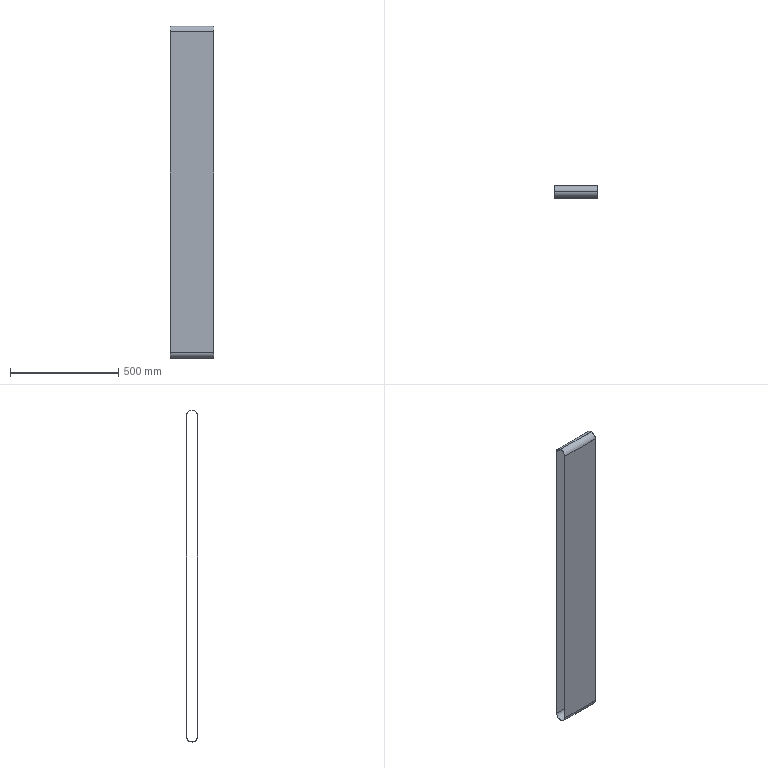Part | STEP file | 02-15 Conveyor belt | 1 solid | 12 faces | box 200 x 54 x 1534 mm | volume 1249345 mm3 | cylinder 6 | plane 6 | commonest cylinder face diameters 50 x3 54 x3
STEP:
#1=CARTESIAN_POINT('',(0.,0.,0.));
#2=DIRECTION('',(0.,0.,1.));
#3=DIRECTION('',(1.,0.,0.));
#4=AXIS2_PLACEMENT_3D('',#1,#2,#3);
#5=CARTESIAN_POINT('',(-100.,25.,740.));
#6=VERTEX_POINT('',#5);
#7=CARTESIAN_POINT('',(100.,25.,740.));
#8=VERTEX_POINT('',#7);
#9=CARTESIAN_POINT('',(0.,25.,740.));
#10=DIRECTION('',(1.,0.,0.));
#11=VECTOR('',#10,1.);
#12=LINE('',#9,#11);
#13=CARTESIAN_POINT('',(100.,0.,740.));
#14=DIRECTION('',(-1.,0.,0.));
#15=DIRECTION('',(0.,0.,1.));
#16=AXIS2_PLACEMENT_3D('',#13,#14,#15);
#17=CYLINDRICAL_SURFACE('',#16,25.);
#18=CARTESIAN_POINT('',(1.571,100.));
#19=DIRECTION('',(0.,-1.));
#20=VECTOR('',#19,1.);
#21=LINE('',#18,#20);
#22=(GEOMETRIC_REPRESENTATION_CONTEXT(2)PARAMETRIC_REPRESENTATION_CONTEXT()REPRESENTATION_CONTEXT('',''));
#23=DEFINITIONAL_REPRESENTATION('',(#21),#22);
#24=PCURVE('',#17,#23);
#25=CARTESIAN_POINT('',(-100.,25.,740.));
#26=DIRECTION('',(0.,-1.,0.));
#27=DIRECTION('',(0.,0.,-1.));
#28=AXIS2_PLACEMENT_3D('',#25,#26,#27);
#29=PLANE('',#28);
#30=CARTESIAN_POINT('',(0.000000005,100.));
#31=DIRECTION('',(0.,1.));
#32=VECTOR('',#31,1.);
#33=LINE('',#30,#32);
#34=(GEOMETRIC_REPRESENTATION_CONTEXT(2)PARAMETRIC_REPRESENTATION_CONTEXT()REPRESENTATION_CONTEXT('',''));
#35=DEFINITIONAL_REPRESENTATION('',(#33),#34);
#36=PCURVE('',#29,#35);
#37=SURFACE_CURVE('',#12,(#24,#36),.PCURVE_S1.);
#38=EDGE_CURVE('',#6,#8,#37,.T.);
#39=ORIENTED_EDGE('',*,*,#38,.F.);
#40=CARTESIAN_POINT('',(-100.,0.,765.));
#41=VERTEX_POINT('',#40);
#42=CARTESIAN_POINT('',(-100.,0.,740.));
#43=DIRECTION('',(-1.,0.,0.));
#44=DIRECTION('',(0.,0.,1.));
#45=AXIS2_PLACEMENT_3D('',#42,#43,#44);
#46=CIRCLE('',#45,25.);
#47=CARTESIAN_POINT('',(0.,200.));
#48=DIRECTION('',(1.,0.));
#49=VECTOR('',#48,1.);
#50=LINE('',#47,#49);
#51=(GEOMETRIC_REPRESENTATION_CONTEXT(2)PARAMETRIC_REPRESENTATION_CONTEXT()REPRESENTATION_CONTEXT('',''));
#52=DEFINITIONAL_REPRESENTATION('',(#50),#51);
#53=PCURVE('',#17,#52);
#54=CARTESIAN_POINT('',(-100.,-27.,776.204));
#55=DIRECTION('',(1.,0.,0.));
#56=DIRECTION('',(0.,0.,-1.));
#57=AXIS2_PLACEMENT_3D('',#54,#55,#56);
#58=PLANE('',#57);
#59=CARTESIAN_POINT('',(11.204,27.));
#60=CARTESIAN_POINT('',(11.204,70.301));
#61=CARTESIAN_POINT('',(48.704,48.651));
#62=CARTESIAN_POINT('',(86.204,27.));
#63=CARTESIAN_POINT('',(48.704,5.349));
#64=CARTESIAN_POINT('',(11.204,-16.301));
#65=CARTESIAN_POINT('',(11.204,27.));
#66=(BOUNDED_CURVE()B_SPLINE_CURVE(2,(#59,#60,#61,#62,#63,#64,#65),.UNSPECIFIED.,.T.,.F.)B_SPLINE_CURVE_WITH_KNOTS((1,2,2,2,2,1),(-2.094,0.,2.094,4.189,6.283,8.378),.UNSPECIFIED.)CURVE()GEOMETRIC_REPRESENTATION_ITEM()RATIONAL_B_SPLINE_CURVE((1.,0.5,1.,0.5,1.,0.5,1.))REPRESENTATION_ITEM(''));
#67=(GEOMETRIC_REPRESENTATION_CONTEXT(2)PARAMETRIC_REPRESENTATION_CONTEXT()REPRESENTATION_CONTEXT('',''));
#68=DEFINITIONAL_REPRESENTATION('',(#66),#67);
#69=PCURVE('',#58,#68);
#70=SURFACE_CURVE('',#46,(#53,#69),.PCURVE_S1.);
#71=EDGE_CURVE('',#41,#6,#70,.T.);
#72=ORIENTED_EDGE('',*,*,#71,.F.);
#73=CARTESIAN_POINT('',(100.,0.,765.));
#74=VERTEX_POINT('',#73);
#75=CARTESIAN_POINT('',(100.,0.,765.));
#76=DIRECTION('',(-1.,0.,0.));
#77=VECTOR('',#76,1.);
#78=LINE('',#75,#77);
#79=CARTESIAN_POINT('',(0.,0.));
#80=DIRECTION('',(0.,1.));
#81=VECTOR('',#80,1.);
#82=LINE('',#79,#81);
#83=(GEOMETRIC_REPRESENTATION_CONTEXT(2)PARAMETRIC_REPRESENTATION_CONTEXT()REPRESENTATION_CONTEXT('',''));
#84=DEFINITIONAL_REPRESENTATION('',(#82),#83);
#85=PCURVE('',#17,#84);
#86=CARTESIAN_POINT('',(100.,0.,740.));
#87=DIRECTION('',(-1.,0.,0.));
#88=DIRECTION('',(0.,0.,1.));
#89=AXIS2_PLACEMENT_3D('',#86,#87,#88);
#90=CYLINDRICAL_SURFACE('',#89,25.);
#91=CARTESIAN_POINT('',(6.283,0.));
#92=DIRECTION('',(0.,1.));
#93=VECTOR('',#92,1.);
#94=LINE('',#91,#93);
#95=(GEOMETRIC_REPRESENTATION_CONTEXT(2)PARAMETRIC_REPRESENTATION_CONTEXT()REPRESENTATION_CONTEXT('',''));
#96=DEFINITIONAL_REPRESENTATION('',(#94),#95);
#97=PCURVE('',#90,#96);
#98=SURFACE_CURVE('',#78,(#85,#97),.PCURVE_S1.);
#99=EDGE_CURVE('',#74,#41,#98,.T.);
#100=ORIENTED_EDGE('',*,*,#99,.F.);
#101=CARTESIAN_POINT('',(100.,0.,740.));
#102=DIRECTION('',(1.,0.,0.));
#103=DIRECTION('',(0.,0.,1.));
#104=AXIS2_PLACEMENT_3D('',#101,#102,#103);
#105=CIRCLE('',#104,25.);
#106=CARTESIAN_POINT('',(6.283,0.));
#107=DIRECTION('',(-1.,0.));
#108=VECTOR('',#107,1.);
#109=LINE('',#106,#108);
#110=(GEOMETRIC_REPRESENTATION_CONTEXT(2)PARAMETRIC_REPRESENTATION_CONTEXT()REPRESENTATION_CONTEXT('',''));
#111=DEFINITIONAL_REPRESENTATION('',(#109),#110);
#112=PCURVE('',#17,#111);
#113=CARTESIAN_POINT('',(100.,-27.,776.204));
#114=DIRECTION('',(1.,0.,0.));
#115=DIRECTION('',(0.,0.,-1.));
#116=AXIS2_PLACEMENT_3D('',#113,#114,#115);
#117=PLANE('',#116);
#118=CARTESIAN_POINT('',(36.204,27.));
#119=DIRECTION('',(-1.,0.));
#120=AXIS2_PLACEMENT_2D('',#118,#119);
#121=CIRCLE('',#120,25.);
#122=(GEOMETRIC_REPRESENTATION_CONTEXT(2)PARAMETRIC_REPRESENTATION_CONTEXT()REPRESENTATION_CONTEXT('',''));
#123=DEFINITIONAL_REPRESENTATION('',(#121),#122);
#124=PCURVE('',#117,#123);
#125=SURFACE_CURVE('',#105,(#112,#124),.PCURVE_S1.);
#126=EDGE_CURVE('',#8,#74,#125,.T.);
#127=ORIENTED_EDGE('',*,*,#126,.F.);
#128=EDGE_LOOP('',(#39,#72,#100,#127));
#129=FACE_BOUND('',#128,.F.);
#130=ADVANCED_FACE('',(#129),#17,.F.);
#131=CARTESIAN_POINT('',(100.,0.,767.));
#132=VERTEX_POINT('',#131);
#133=CARTESIAN_POINT('',(100.,-27.,740.));
#134=VERTEX_POINT('',#133);
#135=CARTESIAN_POINT('',(100.,0.,740.));
#136=DIRECTION('',(1.,0.,0.));
#137=DIRECTION('',(0.,0.,1.));
#138=AXIS2_PLACEMENT_3D('',#135,#136,#137);
#139=CIRCLE('',#138,27.);
#140=CARTESIAN_POINT('',(100.,0.,740.));
#141=DIRECTION('',(-1.,0.,0.));
#142=DIRECTION('',(0.,0.,1.));
#143=AXIS2_PLACEMENT_3D('',#140,#141,#142);
#144=CYLINDRICAL_SURFACE('',#143,27.);
#145=CARTESIAN_POINT('',(6.283,0.));
#146=DIRECTION('',(-1.,0.));
#147=VECTOR('',#146,1.);
#148=LINE('',#145,#147);
#149=(GEOMETRIC_REPRESENTATION_CONTEXT(2)PARAMETRIC_REPRESENTATION_CONTEXT()REPRESENTATION_CONTEXT('',''));
#150=DEFINITIONAL_REPRESENTATION('',(#148),#149);
#151=PCURVE('',#144,#150);
#152=CARTESIAN_POINT('',(36.204,27.));
#153=DIRECTION('',(-1.,0.));
#154=AXIS2_PLACEMENT_2D('',#152,#153);
#155=CIRCLE('',#154,27.);
#156=(GEOMETRIC_REPRESENTATION_CONTEXT(2)PARAMETRIC_REPRESENTATION_CONTEXT()REPRESENTATION_CONTEXT('',''));
#157=DEFINITIONAL_REPRESENTATION('',(#155),#156);
#158=PCURVE('',#117,#157);
#159=SURFACE_CURVE('',#139,(#151,#158),.PCURVE_S1.);
#160=EDGE_CURVE('',#132,#134,#159,.T.);
#161=ORIENTED_EDGE('',*,*,#160,.F.);
#162=CARTESIAN_POINT('',(-100.,0.,767.));
#163=VERTEX_POINT('',#162);
#164=CARTESIAN_POINT('',(100.,0.,767.));
#165=DIRECTION('',(-1.,0.,0.));
#166=VECTOR('',#165,1.);
#167=LINE('',#164,#166);
#168=CARTESIAN_POINT('',(6.283,0.));
#169=DIRECTION('',(0.,1.));
#170=VECTOR('',#169,1.);
#171=LINE('',#168,#170);
#172=(GEOMETRIC_REPRESENTATION_CONTEXT(2)PARAMETRIC_REPRESENTATION_CONTEXT()REPRESENTATION_CONTEXT('',''));
#173=DEFINITIONAL_REPRESENTATION('',(#171),#172);
#174=PCURVE('',#144,#173);
#175=CARTESIAN_POINT('',(100.,0.,740.));
#176=DIRECTION('',(-1.,0.,0.));
#177=DIRECTION('',(0.,0.,1.));
#178=AXIS2_PLACEMENT_3D('',#175,#176,#177);
#179=CYLINDRICAL_SURFACE('',#178,27.);
#180=CARTESIAN_POINT('',(0.,0.));
#181=DIRECTION('',(0.,1.));
#182=VECTOR('',#181,1.);
#183=LINE('',#180,#182);
#184=(GEOMETRIC_REPRESENTATION_CONTEXT(2)PARAMETRIC_REPRESENTATION_CONTEXT()REPRESENTATION_CONTEXT('',''));
#185=DEFINITIONAL_REPRESENTATION('',(#183),#184);
#186=PCURVE('',#179,#185);
#187=SURFACE_CURVE('',#167,(#174,#186),.PCURVE_S1.);
#188=EDGE_CURVE('',#132,#163,#187,.T.);
#189=ORIENTED_EDGE('',*,*,#188,.T.);
#190=CARTESIAN_POINT('',(-100.,-27.,740.));
#191=VERTEX_POINT('',#190);
#192=CARTESIAN_POINT('',(-100.,0.,740.));
#193=DIRECTION('',(1.,0.,0.));
#194=DIRECTION('',(0.,0.,1.));
#195=AXIS2_PLACEMENT_3D('',#192,#193,#194);
#196=CIRCLE('',#195,27.);
#197=CARTESIAN_POINT('',(6.283,200.));
#198=DIRECTION('',(-1.,0.));
#199=VECTOR('',#198,1.);
#200=LINE('',#197,#199);
#201=(GEOMETRIC_REPRESENTATION_CONTEXT(2)PARAMETRIC_REPRESENTATION_CONTEXT()REPRESENTATION_CONTEXT('',''));
#202=DEFINITIONAL_REPRESENTATION('',(#200),#201);
#203=PCURVE('',#144,#202);
#204=CARTESIAN_POINT('',(36.204,27.));
#205=DIRECTION('',(-1.,0.));
#206=AXIS2_PLACEMENT_2D('',#204,#205);
#207=CIRCLE('',#206,27.);
#208=(GEOMETRIC_REPRESENTATION_CONTEXT(2)PARAMETRIC_REPRESENTATION_CONTEXT()REPRESENTATION_CONTEXT('',''));
#209=DEFINITIONAL_REPRESENTATION('',(#207),#208);
#210=PCURVE('',#58,#209);
#211=SURFACE_CURVE('',#196,(#203,#210),.PCURVE_S1.);
#212=EDGE_CURVE('',#163,#191,#211,.T.);
#213=ORIENTED_EDGE('',*,*,#212,.T.);
#214=CARTESIAN_POINT('',(0.,-27.,740.));
#215=DIRECTION('',(1.,0.,0.));
#216=VECTOR('',#215,1.);
#217=LINE('',#214,#216);
#218=CARTESIAN_POINT('',(4.712,100.));
#219=DIRECTION('',(0.,-1.));
#220=VECTOR('',#219,1.);
#221=LINE('',#218,#220);
#222=(GEOMETRIC_REPRESENTATION_CONTEXT(2)PARAMETRIC_REPRESENTATION_CONTEXT()REPRESENTATION_CONTEXT('',''));
#223=DEFINITIONAL_REPRESENTATION('',(#221),#222);
#224=PCURVE('',#144,#223);
#225=CARTESIAN_POINT('',(-100.,-27.,-740.));
#226=DIRECTION('',(0.,1.,0.));
#227=DIRECTION('',(0.,0.,1.));
#228=AXIS2_PLACEMENT_3D('',#225,#226,#227);
#229=PLANE('',#228);
#230=CARTESIAN_POINT('',(1480.,100.));
#231=DIRECTION('',(0.,1.));
#232=VECTOR('',#231,1.);
#233=LINE('',#230,#232);
#234=(GEOMETRIC_REPRESENTATION_CONTEXT(2)PARAMETRIC_REPRESENTATION_CONTEXT()REPRESENTATION_CONTEXT('',''));
#235=DEFINITIONAL_REPRESENTATION('',(#233),#234);
#236=PCURVE('',#229,#235);
#237=SURFACE_CURVE('',#217,(#224,#236),.PCURVE_S1.);
#238=EDGE_CURVE('',#191,#134,#237,.T.);
#239=ORIENTED_EDGE('',*,*,#238,.T.);
#240=EDGE_LOOP('',(#161,#189,#213,#239));
#241=FACE_BOUND('',#240,.T.);
#242=ADVANCED_FACE('',(#241),#144,.T.);
#243=CARTESIAN_POINT('',(-100.,-25.,740.));
#244=VERTEX_POINT('',#243);
#245=CARTESIAN_POINT('',(-100.,0.,740.));
#246=DIRECTION('',(-1.,0.,0.));
#247=DIRECTION('',(0.,0.,1.));
#248=AXIS2_PLACEMENT_3D('',#245,#246,#247);
#249=CIRCLE('',#248,25.);
#250=CARTESIAN_POINT('',(0.,200.));
#251=DIRECTION('',(1.,0.));
#252=VECTOR('',#251,1.);
#253=LINE('',#250,#252);
#254=(GEOMETRIC_REPRESENTATION_CONTEXT(2)PARAMETRIC_REPRESENTATION_CONTEXT()REPRESENTATION_CONTEXT('',''));
#255=DEFINITIONAL_REPRESENTATION('',(#253),#254);
#256=PCURVE('',#90,#255);
#257=CARTESIAN_POINT('',(11.204,27.));
#258=CARTESIAN_POINT('',(11.204,70.301));
#259=CARTESIAN_POINT('',(48.704,48.651));
#260=CARTESIAN_POINT('',(86.204,27.));
#261=CARTESIAN_POINT('',(48.704,5.349));
#262=CARTESIAN_POINT('',(11.204,-16.301));
#263=CARTESIAN_POINT('',(11.204,27.));
#264=(BOUNDED_CURVE()B_SPLINE_CURVE(2,(#257,#258,#259,#260,#261,#262,#263),.UNSPECIFIED.,.T.,.F.)B_SPLINE_CURVE_WITH_KNOTS((1,2,2,2,2,1),(-2.094,0.,2.094,4.189,6.283,8.378),.UNSPECIFIED.)CURVE()GEOMETRIC_REPRESENTATION_ITEM()RATIONAL_B_SPLINE_CURVE((1.,0.5,1.,0.5,1.,0.5,1.))REPRESENTATION_ITEM(''));
#265=(GEOMETRIC_REPRESENTATION_CONTEXT(2)PARAMETRIC_REPRESENTATION_CONTEXT()REPRESENTATION_CONTEXT('',''));
#266=DEFINITIONAL_REPRESENTATION('',(#264),#265);
#267=PCURVE('',#58,#266);
#268=SURFACE_CURVE('',#249,(#256,#267),.PCURVE_S1.);
#269=EDGE_CURVE('',#244,#41,#268,.T.);
#270=ORIENTED_EDGE('',*,*,#269,.F.);
#271=CARTESIAN_POINT('',(100.,-25.,740.));
#272=VERTEX_POINT('',#271);
#273=CARTESIAN_POINT('',(0.,-25.,740.));
#274=DIRECTION('',(-1.,0.,0.));
#275=VECTOR('',#274,1.);
#276=LINE('',#273,#275);
#277=CARTESIAN_POINT('',(4.712,100.));
#278=DIRECTION('',(0.,1.));
#279=VECTOR('',#278,1.);
#280=LINE('',#277,#279);
#281=(GEOMETRIC_REPRESENTATION_CONTEXT(2)PARAMETRIC_REPRESENTATION_CONTEXT()REPRESENTATION_CONTEXT('',''));
#282=DEFINITIONAL_REPRESENTATION('',(#280),#281);
#283=PCURVE('',#90,#282);
#284=CARTESIAN_POINT('',(-100.,-25.,-740.));
#285=DIRECTION('',(0.,1.,0.));
#286=DIRECTION('',(0.,0.,1.));
#287=AXIS2_PLACEMENT_3D('',#284,#285,#286);
#288=PLANE('',#287);
#289=CARTESIAN_POINT('',(1480.,100.));
#290=DIRECTION('',(0.,-1.));
#291=VECTOR('',#290,1.);
#292=LINE('',#289,#291);
#293=(GEOMETRIC_REPRESENTATION_CONTEXT(2)PARAMETRIC_REPRESENTATION_CONTEXT()REPRESENTATION_CONTEXT('',''));
#294=DEFINITIONAL_REPRESENTATION('',(#292),#293);
#295=PCURVE('',#288,#294);
#296=SURFACE_CURVE('',#276,(#283,#295),.PCURVE_S1.);
#297=EDGE_CURVE('',#272,#244,#296,.T.);
#298=ORIENTED_EDGE('',*,*,#297,.F.);
#299=CARTESIAN_POINT('',(100.,0.,740.));
#300=DIRECTION('',(1.,0.,0.));
#301=DIRECTION('',(0.,0.,1.));
#302=AXIS2_PLACEMENT_3D('',#299,#300,#301);
#303=CIRCLE('',#302,25.);
#304=CARTESIAN_POINT('',(6.283,0.));
#305=DIRECTION('',(-1.,0.));
#306=VECTOR('',#305,1.);
#307=LINE('',#304,#306);
#308=(GEOMETRIC_REPRESENTATION_CONTEXT(2)PARAMETRIC_REPRESENTATION_CONTEXT()REPRESENTATION_CONTEXT('',''));
#309=DEFINITIONAL_REPRESENTATION('',(#307),#308);
#310=PCURVE('',#90,#309);
#311=CARTESIAN_POINT('',(36.204,27.));
#312=DIRECTION('',(-1.,0.));
#313=AXIS2_PLACEMENT_2D('',#311,#312);
#314=CIRCLE('',#313,25.);
#315=(GEOMETRIC_REPRESENTATION_CONTEXT(2)PARAMETRIC_REPRESENTATION_CONTEXT()REPRESENTATION_CONTEXT('',''));
#316=DEFINITIONAL_REPRESENTATION('',(#314),#315);
#317=PCURVE('',#117,#316);
#318=SURFACE_CURVE('',#303,(#310,#317),.PCURVE_S1.);
#319=EDGE_CURVE('',#74,#272,#318,.T.);
#320=ORIENTED_EDGE('',*,*,#319,.F.);
#321=ORIENTED_EDGE('',*,*,#99,.T.);
#322=EDGE_LOOP('',(#270,#298,#320,#321));
#323=FACE_BOUND('',#322,.F.);
#324=ADVANCED_FACE('',(#323),#90,.F.);
#325=CARTESIAN_POINT('',(100.,25.,-740.));
#326=VERTEX_POINT('',#325);
#327=CARTESIAN_POINT('',(100.,25.,0.));
#328=DIRECTION('',(0.,0.,1.));
#329=VECTOR('',#328,1.);
#330=LINE('',#327,#329);
#331=CARTESIAN_POINT('',(740.,200.));
#332=DIRECTION('',(-1.,0.));
#333=VECTOR('',#332,1.);
#334=LINE('',#331,#333);
#335=(GEOMETRIC_REPRESENTATION_CONTEXT(2)PARAMETRIC_REPRESENTATION_CONTEXT()REPRESENTATION_CONTEXT('',''));
#336=DEFINITIONAL_REPRESENTATION('',(#334),#335);
#337=PCURVE('',#29,#336);
#338=CARTESIAN_POINT('',(776.204,52.));
#339=DIRECTION('',(-1.,0.));
#340=VECTOR('',#339,1.);
#341=LINE('',#338,#340);
#342=(GEOMETRIC_REPRESENTATION_CONTEXT(2)PARAMETRIC_REPRESENTATION_CONTEXT()REPRESENTATION_CONTEXT('',''));
#343=DEFINITIONAL_REPRESENTATION('',(#341),#342);
#344=PCURVE('',#117,#343);
#345=SURFACE_CURVE('',#330,(#337,#344),.PCURVE_S1.);
#346=EDGE_CURVE('',#326,#8,#345,.T.);
#347=ORIENTED_EDGE('',*,*,#346,.T.);
#348=ORIENTED_EDGE('',*,*,#38,.F.);
#349=CARTESIAN_POINT('',(-100.,25.,-740.));
#350=VERTEX_POINT('',#349);
#351=CARTESIAN_POINT('',(-100.,25.,0.));
#352=DIRECTION('',(0.,0.,-1.));
#353=VECTOR('',#352,1.);
#354=LINE('',#351,#353);
#355=CARTESIAN_POINT('',(740.,0.));
#356=DIRECTION('',(1.,0.));
#357=VECTOR('',#356,1.);
#358=LINE('',#355,#357);
#359=(GEOMETRIC_REPRESENTATION_CONTEXT(2)PARAMETRIC_REPRESENTATION_CONTEXT()REPRESENTATION_CONTEXT('',''));
#360=DEFINITIONAL_REPRESENTATION('',(#358),#359);
#361=PCURVE('',#29,#360);
#362=CARTESIAN_POINT('',(776.204,52.));
#363=DIRECTION('',(1.,0.));
#364=VECTOR('',#363,1.);
#365=LINE('',#362,#364);
#366=(GEOMETRIC_REPRESENTATION_CONTEXT(2)PARAMETRIC_REPRESENTATION_CONTEXT()REPRESENTATION_CONTEXT('',''));
#367=DEFINITIONAL_REPRESENTATION('',(#365),#366);
#368=PCURVE('',#58,#367);
#369=SURFACE_CURVE('',#354,(#361,#368),.PCURVE_S1.);
#370=EDGE_CURVE('',#6,#350,#369,.T.);
#371=ORIENTED_EDGE('',*,*,#370,.T.);
#372=CARTESIAN_POINT('',(0.,25.,-740.));
#373=DIRECTION('',(1.,0.,0.));
#374=VECTOR('',#373,1.);
#375=LINE('',#372,#374);
#376=CARTESIAN_POINT('',(1480.,100.));
#377=DIRECTION('',(0.,1.));
#378=VECTOR('',#377,1.);
#379=LINE('',#376,#378);
#380=(GEOMETRIC_REPRESENTATION_CONTEXT(2)PARAMETRIC_REPRESENTATION_CONTEXT()REPRESENTATION_CONTEXT('',''));
#381=DEFINITIONAL_REPRESENTATION('',(#379),#380);
#382=PCURVE('',#29,#381);
#383=CARTESIAN_POINT('',(100.,0.,-740.));
#384=DIRECTION('',(-1.,0.,0.));
#385=DIRECTION('',(0.,0.,1.));
#386=AXIS2_PLACEMENT_3D('',#383,#384,#385);
#387=CYLINDRICAL_SURFACE('',#386,25.);
#388=CARTESIAN_POINT('',(1.571,100.));
#389=DIRECTION('',(0.,-1.));
#390=VECTOR('',#389,1.);
#391=LINE('',#388,#390);
#392=(GEOMETRIC_REPRESENTATION_CONTEXT(2)PARAMETRIC_REPRESENTATION_CONTEXT()REPRESENTATION_CONTEXT('',''));
#393=DEFINITIONAL_REPRESENTATION('',(#391),#392);
#394=PCURVE('',#387,#393);
#395=SURFACE_CURVE('',#375,(#382,#394),.PCURVE_S1.);
#396=EDGE_CURVE('',#350,#326,#395,.T.);
#397=ORIENTED_EDGE('',*,*,#396,.T.);
#398=EDGE_LOOP('',(#347,#348,#371,#397));
#399=FACE_BOUND('',#398,.T.);
#400=ADVANCED_FACE('',(#399),#29,.T.);
#401=ORIENTED_EDGE('',*,*,#269,.F.);
#402=CARTESIAN_POINT('',(-100.,-25.,-740.));
#403=VERTEX_POINT('',#402);
#404=CARTESIAN_POINT('',(-100.,-25.,0.));
#405=DIRECTION('',(0.,0.,1.));
#406=VECTOR('',#405,1.);
#407=LINE('',#404,#406);
#408=CARTESIAN_POINT('',(776.204,2.));
#409=DIRECTION('',(-1.,0.));
#410=VECTOR('',#409,1.);
#411=LINE('',#408,#410);
#412=(GEOMETRIC_REPRESENTATION_CONTEXT(2)PARAMETRIC_REPRESENTATION_CONTEXT()REPRESENTATION_CONTEXT('',''));
#413=DEFINITIONAL_REPRESENTATION('',(#411),#412);
#414=PCURVE('',#58,#413);
#415=CARTESIAN_POINT('',(740.,0.));
#416=DIRECTION('',(1.,0.));
#417=VECTOR('',#416,1.);
#418=LINE('',#415,#417);
#419=(GEOMETRIC_REPRESENTATION_CONTEXT(2)PARAMETRIC_REPRESENTATION_CONTEXT()REPRESENTATION_CONTEXT('',''));
#420=DEFINITIONAL_REPRESENTATION('',(#418),#419);
#421=PCURVE('',#288,#420);
#422=SURFACE_CURVE('',#407,(#414,#421),.PCURVE_S1.);
#423=EDGE_CURVE('',#403,#244,#422,.T.);
#424=ORIENTED_EDGE('',*,*,#423,.F.);
#425=CARTESIAN_POINT('',(-100.,0.,-740.));
#426=DIRECTION('',(-1.,0.,0.));
#427=DIRECTION('',(0.,0.,1.));
#428=AXIS2_PLACEMENT_3D('',#425,#426,#427);
#429=CIRCLE('',#428,25.);
#430=CARTESIAN_POINT('',(1491.204,27.));
#431=CARTESIAN_POINT('',(1491.204,70.301));
#432=CARTESIAN_POINT('',(1528.704,48.651));
#433=CARTESIAN_POINT('',(1566.204,27.));
#434=CARTESIAN_POINT('',(1528.704,5.349));
#435=CARTESIAN_POINT('',(1491.204,-16.301));
#436=CARTESIAN_POINT('',(1491.204,27.));
#437=(BOUNDED_CURVE()B_SPLINE_CURVE(2,(#430,#431,#432,#433,#434,#435,#436),.UNSPECIFIED.,.T.,.F.)B_SPLINE_CURVE_WITH_KNOTS((1,2,2,2,2,1),(-2.094,0.,2.094,4.189,6.283,8.378),.UNSPECIFIED.)CURVE()GEOMETRIC_REPRESENTATION_ITEM()RATIONAL_B_SPLINE_CURVE((1.,0.5,1.,0.5,1.,0.5,1.))REPRESENTATION_ITEM(''));
#438=(GEOMETRIC_REPRESENTATION_CONTEXT(2)PARAMETRIC_REPRESENTATION_CONTEXT()REPRESENTATION_CONTEXT('',''));
#439=DEFINITIONAL_REPRESENTATION('',(#437),#438);
#440=PCURVE('',#58,#439);
#441=CARTESIAN_POINT('',(0.,200.));
#442=DIRECTION('',(1.,0.));
#443=VECTOR('',#442,1.);
#444=LINE('',#441,#443);
#445=(GEOMETRIC_REPRESENTATION_CONTEXT(2)PARAMETRIC_REPRESENTATION_CONTEXT()REPRESENTATION_CONTEXT('',''));
#446=DEFINITIONAL_REPRESENTATION('',(#444),#445);
#447=PCURVE('',#387,#446);
#448=SURFACE_CURVE('',#429,(#440,#447),.PCURVE_S1.);
#449=EDGE_CURVE('',#350,#403,#448,.T.);
#450=ORIENTED_EDGE('',*,*,#449,.F.);
#451=ORIENTED_EDGE('',*,*,#370,.F.);
#452=ORIENTED_EDGE('',*,*,#71,.F.);
#453=EDGE_LOOP('',(#401,#424,#450,#451,#452));
#454=FACE_BOUND('',#453,.T.);
#455=CARTESIAN_POINT('',(-100.,27.,-740.));
#456=VERTEX_POINT('',#455);
#457=CARTESIAN_POINT('',(-100.,27.,740.));
#458=VERTEX_POINT('',#457);
#459=CARTESIAN_POINT('',(-100.,27.,0.));
#460=DIRECTION('',(0.,0.,1.));
#461=VECTOR('',#460,1.);
#462=LINE('',#459,#461);
#463=CARTESIAN_POINT('',(776.204,54.));
#464=DIRECTION('',(-1.,0.));
#465=VECTOR('',#464,1.);
#466=LINE('',#463,#465);
#467=(GEOMETRIC_REPRESENTATION_CONTEXT(2)PARAMETRIC_REPRESENTATION_CONTEXT()REPRESENTATION_CONTEXT('',''));
#468=DEFINITIONAL_REPRESENTATION('',(#466),#467);
#469=PCURVE('',#58,#468);
#470=CARTESIAN_POINT('',(-100.,27.,740.));
#471=DIRECTION('',(0.,-1.,0.));
#472=DIRECTION('',(0.,0.,-1.));
#473=AXIS2_PLACEMENT_3D('',#470,#471,#472);
#474=PLANE('',#473);
#475=CARTESIAN_POINT('',(740.,0.));
#476=DIRECTION('',(-1.,0.));
#477=VECTOR('',#476,1.);
#478=LINE('',#475,#477);
#479=(GEOMETRIC_REPRESENTATION_CONTEXT(2)PARAMETRIC_REPRESENTATION_CONTEXT()REPRESENTATION_CONTEXT('',''));
#480=DEFINITIONAL_REPRESENTATION('',(#478),#479);
#481=PCURVE('',#474,#480);
#482=SURFACE_CURVE('',#462,(#469,#481),.PCURVE_S1.);
#483=EDGE_CURVE('',#456,#458,#482,.T.);
#484=ORIENTED_EDGE('',*,*,#483,.F.);
#485=CARTESIAN_POINT('',(-100.,-27.,-740.));
#486=VERTEX_POINT('',#485);
#487=CARTESIAN_POINT('',(-100.,0.,-740.));
#488=DIRECTION('',(1.,0.,0.));
#489=DIRECTION('',(0.,0.,1.));
#490=AXIS2_PLACEMENT_3D('',#487,#488,#489);
#491=CIRCLE('',#490,27.);
#492=CARTESIAN_POINT('',(1516.204,27.));
#493=DIRECTION('',(-1.,0.));
#494=AXIS2_PLACEMENT_2D('',#492,#493);
#495=CIRCLE('',#494,27.);
#496=(GEOMETRIC_REPRESENTATION_CONTEXT(2)PARAMETRIC_REPRESENTATION_CONTEXT()REPRESENTATION_CONTEXT('',''));
#497=DEFINITIONAL_REPRESENTATION('',(#495),#496);
#498=PCURVE('',#58,#497);
#499=CARTESIAN_POINT('',(100.,0.,-740.));
#500=DIRECTION('',(-1.,0.,0.));
#501=DIRECTION('',(0.,0.,1.));
#502=AXIS2_PLACEMENT_3D('',#499,#500,#501);
#503=CYLINDRICAL_SURFACE('',#502,27.);
#504=CARTESIAN_POINT('',(6.283,200.));
#505=DIRECTION('',(-1.,0.));
#506=VECTOR('',#505,1.);
#507=LINE('',#504,#506);
#508=(GEOMETRIC_REPRESENTATION_CONTEXT(2)PARAMETRIC_REPRESENTATION_CONTEXT()REPRESENTATION_CONTEXT('',''));
#509=DEFINITIONAL_REPRESENTATION('',(#507),#508);
#510=PCURVE('',#503,#509);
#511=SURFACE_CURVE('',#491,(#498,#510),.PCURVE_S1.);
#512=EDGE_CURVE('',#486,#456,#511,.T.);
#513=ORIENTED_EDGE('',*,*,#512,.F.);
#514=CARTESIAN_POINT('',(-100.,-27.,0.));
#515=DIRECTION('',(0.,0.,-1.));
#516=VECTOR('',#515,1.);
#517=LINE('',#514,#516);
#518=CARTESIAN_POINT('',(776.204,0.));
#519=DIRECTION('',(1.,0.));
#520=VECTOR('',#519,1.);
#521=LINE('',#518,#520);
#522=(GEOMETRIC_REPRESENTATION_CONTEXT(2)PARAMETRIC_REPRESENTATION_CONTEXT()REPRESENTATION_CONTEXT('',''));
#523=DEFINITIONAL_REPRESENTATION('',(#521),#522);
#524=PCURVE('',#58,#523);
#525=CARTESIAN_POINT('',(740.,0.));
#526=DIRECTION('',(-1.,0.));
#527=VECTOR('',#526,1.);
#528=LINE('',#525,#527);
#529=(GEOMETRIC_REPRESENTATION_CONTEXT(2)PARAMETRIC_REPRESENTATION_CONTEXT()REPRESENTATION_CONTEXT('',''));
#530=DEFINITIONAL_REPRESENTATION('',(#528),#529);
#531=PCURVE('',#229,#530);
#532=SURFACE_CURVE('',#517,(#524,#531),.PCURVE_S1.);
#533=EDGE_CURVE('',#191,#486,#532,.T.);
#534=ORIENTED_EDGE('',*,*,#533,.F.);
#535=ORIENTED_EDGE('',*,*,#212,.F.);
#536=CARTESIAN_POINT('',(-100.,0.,740.));
#537=DIRECTION('',(1.,0.,0.));
#538=DIRECTION('',(0.,0.,1.));
#539=AXIS2_PLACEMENT_3D('',#536,#537,#538);
#540=CIRCLE('',#539,27.);
#541=CARTESIAN_POINT('',(36.204,27.));
#542=DIRECTION('',(-1.,0.));
#543=AXIS2_PLACEMENT_2D('',#541,#542);
#544=CIRCLE('',#543,27.);
#545=(GEOMETRIC_REPRESENTATION_CONTEXT(2)PARAMETRIC_REPRESENTATION_CONTEXT()REPRESENTATION_CONTEXT('',''));
#546=DEFINITIONAL_REPRESENTATION('',(#544),#545);
#547=PCURVE('',#58,#546);
#548=CARTESIAN_POINT('',(6.283,200.));
#549=DIRECTION('',(-1.,0.));
#550=VECTOR('',#549,1.);
#551=LINE('',#548,#550);
#552=(GEOMETRIC_REPRESENTATION_CONTEXT(2)PARAMETRIC_REPRESENTATION_CONTEXT()REPRESENTATION_CONTEXT('',''));
#553=DEFINITIONAL_REPRESENTATION('',(#551),#552);
#554=PCURVE('',#179,#553);
#555=SURFACE_CURVE('',#540,(#547,#554),.PCURVE_S1.);
#556=EDGE_CURVE('',#458,#163,#555,.T.);
#557=ORIENTED_EDGE('',*,*,#556,.F.);
#558=EDGE_LOOP('',(#484,#513,#534,#535,#557));
#559=FACE_BOUND('',#558,.T.);
#560=ADVANCED_FACE('',(#454,#559),#58,.F.);
#561=ORIENTED_EDGE('',*,*,#346,.F.);
#562=CARTESIAN_POINT('',(100.,-25.,-740.));
#563=VERTEX_POINT('',#562);
#564=CARTESIAN_POINT('',(100.,0.,-740.));
#565=DIRECTION('',(-1.,0.,0.));
#566=DIRECTION('',(0.,0.,1.));
#567=AXIS2_PLACEMENT_3D('',#564,#565,#566);
#568=CIRCLE('',#567,25.);
#569=CARTESIAN_POINT('',(1491.204,27.));
#570=CARTESIAN_POINT('',(1491.204,70.301));
#571=CARTESIAN_POINT('',(1528.704,48.651));
#572=CARTESIAN_POINT('',(1566.204,27.));
#573=CARTESIAN_POINT('',(1528.704,5.349));
#574=CARTESIAN_POINT('',(1491.204,-16.301));
#575=CARTESIAN_POINT('',(1491.204,27.));
#576=(BOUNDED_CURVE()B_SPLINE_CURVE(2,(#569,#570,#571,#572,#573,#574,#575),.UNSPECIFIED.,.T.,.F.)B_SPLINE_CURVE_WITH_KNOTS((1,2,2,2,2,1),(-2.094,0.,2.094,4.189,6.283,8.378),.UNSPECIFIED.)CURVE()GEOMETRIC_REPRESENTATION_ITEM()RATIONAL_B_SPLINE_CURVE((1.,0.5,1.,0.5,1.,0.5,1.))REPRESENTATION_ITEM(''));
#577=(GEOMETRIC_REPRESENTATION_CONTEXT(2)PARAMETRIC_REPRESENTATION_CONTEXT()REPRESENTATION_CONTEXT('',''));
#578=DEFINITIONAL_REPRESENTATION('',(#576),#577);
#579=PCURVE('',#117,#578);
#580=CARTESIAN_POINT('',(0.,0.));
#581=DIRECTION('',(1.,0.));
#582=VECTOR('',#581,1.);
#583=LINE('',#580,#582);
#584=(GEOMETRIC_REPRESENTATION_CONTEXT(2)PARAMETRIC_REPRESENTATION_CONTEXT()REPRESENTATION_CONTEXT('',''));
#585=DEFINITIONAL_REPRESENTATION('',(#583),#584);
#586=PCURVE('',#387,#585);
#587=SURFACE_CURVE('',#568,(#579,#586),.PCURVE_S1.);
#588=EDGE_CURVE('',#326,#563,#587,.T.);
#589=ORIENTED_EDGE('',*,*,#588,.T.);
#590=CARTESIAN_POINT('',(100.,-25.,0.));
#591=DIRECTION('',(0.,0.,1.));
#592=VECTOR('',#591,1.);
#593=LINE('',#590,#592);
#594=CARTESIAN_POINT('',(776.204,2.));
#595=DIRECTION('',(-1.,0.));
#596=VECTOR('',#595,1.);
#597=LINE('',#594,#596);
#598=(GEOMETRIC_REPRESENTATION_CONTEXT(2)PARAMETRIC_REPRESENTATION_CONTEXT()REPRESENTATION_CONTEXT('',''));
#599=DEFINITIONAL_REPRESENTATION('',(#597),#598);
#600=PCURVE('',#117,#599);
#601=CARTESIAN_POINT('',(740.,200.));
#602=DIRECTION('',(1.,0.));
#603=VECTOR('',#602,1.);
#604=LINE('',#601,#603);
#605=(GEOMETRIC_REPRESENTATION_CONTEXT(2)PARAMETRIC_REPRESENTATION_CONTEXT()REPRESENTATION_CONTEXT('',''));
#606=DEFINITIONAL_REPRESENTATION('',(#604),#605);
#607=PCURVE('',#288,#606);
#608=SURFACE_CURVE('',#593,(#600,#607),.PCURVE_S1.);
#609=EDGE_CURVE('',#563,#272,#608,.T.);
#610=ORIENTED_EDGE('',*,*,#609,.T.);
#611=ORIENTED_EDGE('',*,*,#319,.F.);
#612=ORIENTED_EDGE('',*,*,#126,.F.);
#613=EDGE_LOOP('',(#561,#589,#610,#611,#612));
#614=FACE_BOUND('',#613,.T.);
#615=CARTESIAN_POINT('',(100.,-27.,-740.));
#616=VERTEX_POINT('',#615);
#617=CARTESIAN_POINT('',(100.,27.,-740.));
#618=VERTEX_POINT('',#617);
#619=CARTESIAN_POINT('',(100.,0.,-740.));
#620=DIRECTION('',(1.,0.,0.));
#621=DIRECTION('',(0.,0.,1.));
#622=AXIS2_PLACEMENT_3D('',#619,#620,#621);
#623=CIRCLE('',#622,27.);
#624=CARTESIAN_POINT('',(1516.204,27.));
#625=DIRECTION('',(-1.,0.));
#626=AXIS2_PLACEMENT_2D('',#624,#625);
#627=CIRCLE('',#626,27.);
#628=(GEOMETRIC_REPRESENTATION_CONTEXT(2)PARAMETRIC_REPRESENTATION_CONTEXT()REPRESENTATION_CONTEXT('',''));
#629=DEFINITIONAL_REPRESENTATION('',(#627),#628);
#630=PCURVE('',#117,#629);
#631=CARTESIAN_POINT('',(6.283,0.));
#632=DIRECTION('',(-1.,0.));
#633=VECTOR('',#632,1.);
#634=LINE('',#631,#633);
#635=(GEOMETRIC_REPRESENTATION_CONTEXT(2)PARAMETRIC_REPRESENTATION_CONTEXT()REPRESENTATION_CONTEXT('',''));
#636=DEFINITIONAL_REPRESENTATION('',(#634),#635);
#637=PCURVE('',#503,#636);
#638=SURFACE_CURVE('',#623,(#630,#637),.PCURVE_S1.);
#639=EDGE_CURVE('',#616,#618,#638,.T.);
#640=ORIENTED_EDGE('',*,*,#639,.T.);
#641=CARTESIAN_POINT('',(100.,27.,740.));
#642=VERTEX_POINT('',#641);
#643=CARTESIAN_POINT('',(100.,27.,0.));
#644=DIRECTION('',(0.,0.,1.));
#645=VECTOR('',#644,1.);
#646=LINE('',#643,#645);
#647=CARTESIAN_POINT('',(776.204,54.));
#648=DIRECTION('',(-1.,0.));
#649=VECTOR('',#648,1.);
#650=LINE('',#647,#649);
#651=(GEOMETRIC_REPRESENTATION_CONTEXT(2)PARAMETRIC_REPRESENTATION_CONTEXT()REPRESENTATION_CONTEXT('',''));
#652=DEFINITIONAL_REPRESENTATION('',(#650),#651);
#653=PCURVE('',#117,#652);
#654=CARTESIAN_POINT('',(740.,200.));
#655=DIRECTION('',(-1.,0.));
#656=VECTOR('',#655,1.);
#657=LINE('',#654,#656);
#658=(GEOMETRIC_REPRESENTATION_CONTEXT(2)PARAMETRIC_REPRESENTATION_CONTEXT()REPRESENTATION_CONTEXT('',''));
#659=DEFINITIONAL_REPRESENTATION('',(#657),#658);
#660=PCURVE('',#474,#659);
#661=SURFACE_CURVE('',#646,(#653,#660),.PCURVE_S1.);
#662=EDGE_CURVE('',#618,#642,#661,.T.);
#663=ORIENTED_EDGE('',*,*,#662,.T.);
#664=CARTESIAN_POINT('',(100.,0.,740.));
#665=DIRECTION('',(1.,0.,0.));
#666=DIRECTION('',(0.,0.,1.));
#667=AXIS2_PLACEMENT_3D('',#664,#665,#666);
#668=CIRCLE('',#667,27.);
#669=CARTESIAN_POINT('',(36.204,27.));
#670=DIRECTION('',(-1.,0.));
#671=AXIS2_PLACEMENT_2D('',#669,#670);
#672=CIRCLE('',#671,27.);
#673=(GEOMETRIC_REPRESENTATION_CONTEXT(2)PARAMETRIC_REPRESENTATION_CONTEXT()REPRESENTATION_CONTEXT('',''));
#674=DEFINITIONAL_REPRESENTATION('',(#672),#673);
#675=PCURVE('',#117,#674);
#676=CARTESIAN_POINT('',(6.283,0.));
#677=DIRECTION('',(-1.,0.));
#678=VECTOR('',#677,1.);
#679=LINE('',#676,#678);
#680=(GEOMETRIC_REPRESENTATION_CONTEXT(2)PARAMETRIC_REPRESENTATION_CONTEXT()REPRESENTATION_CONTEXT('',''));
#681=DEFINITIONAL_REPRESENTATION('',(#679),#680);
#682=PCURVE('',#179,#681);
#683=SURFACE_CURVE('',#668,(#675,#682),.PCURVE_S1.);
#684=EDGE_CURVE('',#642,#132,#683,.T.);
#685=ORIENTED_EDGE('',*,*,#684,.T.);
#686=ORIENTED_EDGE('',*,*,#160,.T.);
#687=CARTESIAN_POINT('',(100.,-27.,0.));
#688=DIRECTION('',(0.,0.,-1.));
#689=VECTOR('',#688,1.);
#690=LINE('',#687,#689);
#691=CARTESIAN_POINT('',(776.204,0.));
#692=DIRECTION('',(1.,0.));
#693=VECTOR('',#692,1.);
#694=LINE('',#691,#693);
#695=(GEOMETRIC_REPRESENTATION_CONTEXT(2)PARAMETRIC_REPRESENTATION_CONTEXT()REPRESENTATION_CONTEXT('',''));
#696=DEFINITIONAL_REPRESENTATION('',(#694),#695);
#697=PCURVE('',#117,#696);
#698=CARTESIAN_POINT('',(740.,200.));
#699=DIRECTION('',(-1.,0.));
#700=VECTOR('',#699,1.);
#701=LINE('',#698,#700);
#702=(GEOMETRIC_REPRESENTATION_CONTEXT(2)PARAMETRIC_REPRESENTATION_CONTEXT()REPRESENTATION_CONTEXT('',''));
#703=DEFINITIONAL_REPRESENTATION('',(#701),#702);
#704=PCURVE('',#229,#703);
#705=SURFACE_CURVE('',#690,(#697,#704),.PCURVE_S1.);
#706=EDGE_CURVE('',#134,#616,#705,.T.);
#707=ORIENTED_EDGE('',*,*,#706,.T.);
#708=EDGE_LOOP('',(#640,#663,#685,#686,#707));
#709=FACE_BOUND('',#708,.T.);
#710=ADVANCED_FACE('',(#614,#709),#117,.T.);
#711=CARTESIAN_POINT('',(0.,-25.,-740.));
#712=DIRECTION('',(1.,0.,0.));
#713=VECTOR('',#712,1.);
#714=LINE('',#711,#713);
#715=CARTESIAN_POINT('',(4.712,100.));
#716=DIRECTION('',(0.,-1.));
#717=VECTOR('',#716,1.);
#718=LINE('',#715,#717);
#719=(GEOMETRIC_REPRESENTATION_CONTEXT(2)PARAMETRIC_REPRESENTATION_CONTEXT()REPRESENTATION_CONTEXT('',''));
#720=DEFINITIONAL_REPRESENTATION('',(#718),#719);
#721=PCURVE('',#387,#720);
#722=CARTESIAN_POINT('',(-0.00000001,100.));
#723=DIRECTION('',(0.,1.));
#724=VECTOR('',#723,1.);
#725=LINE('',#722,#724);
#726=(GEOMETRIC_REPRESENTATION_CONTEXT(2)PARAMETRIC_REPRESENTATION_CONTEXT()REPRESENTATION_CONTEXT('',''));
#727=DEFINITIONAL_REPRESENTATION('',(#725),#726);
#728=PCURVE('',#288,#727);
#729=SURFACE_CURVE('',#714,(#721,#728),.PCURVE_S1.);
#730=EDGE_CURVE('',#403,#563,#729,.T.);
#731=ORIENTED_EDGE('',*,*,#730,.F.);
#732=ORIENTED_EDGE('',*,*,#449,.F.);
#733=ORIENTED_EDGE('',*,*,#396,.T.);
#734=ORIENTED_EDGE('',*,*,#588,.T.);
#735=EDGE_LOOP('',(#731,#732,#733,#734));
#736=FACE_BOUND('',#735,.F.);
#737=ADVANCED_FACE('',(#736),#387,.F.);
#738=ORIENTED_EDGE('',*,*,#609,.F.);
#739=ORIENTED_EDGE('',*,*,#730,.F.);
#740=ORIENTED_EDGE('',*,*,#423,.T.);
#741=ORIENTED_EDGE('',*,*,#297,.F.);
#742=EDGE_LOOP('',(#738,#739,#740,#741));
#743=FACE_BOUND('',#742,.T.);
#744=ADVANCED_FACE('',(#743),#288,.T.);
#745=ORIENTED_EDGE('',*,*,#188,.F.);
#746=ORIENTED_EDGE('',*,*,#684,.F.);
#747=CARTESIAN_POINT('',(0.,27.,740.));
#748=DIRECTION('',(1.,0.,0.));
#749=VECTOR('',#748,1.);
#750=LINE('',#747,#749);
#751=CARTESIAN_POINT('',(1.571,100.));
#752=DIRECTION('',(0.,-1.));
#753=VECTOR('',#752,1.);
#754=LINE('',#751,#753);
#755=(GEOMETRIC_REPRESENTATION_CONTEXT(2)PARAMETRIC_REPRESENTATION_CONTEXT()REPRESENTATION_CONTEXT('',''));
#756=DEFINITIONAL_REPRESENTATION('',(#754),#755);
#757=PCURVE('',#179,#756);
#758=CARTESIAN_POINT('',(0.000000006,100.));
#759=DIRECTION('',(0.,1.));
#760=VECTOR('',#759,1.);
#761=LINE('',#758,#760);
#762=(GEOMETRIC_REPRESENTATION_CONTEXT(2)PARAMETRIC_REPRESENTATION_CONTEXT()REPRESENTATION_CONTEXT('',''));
#763=DEFINITIONAL_REPRESENTATION('',(#761),#762);
#764=PCURVE('',#474,#763);
#765=SURFACE_CURVE('',#750,(#757,#764),.PCURVE_S1.);
#766=EDGE_CURVE('',#458,#642,#765,.T.);
#767=ORIENTED_EDGE('',*,*,#766,.F.);
#768=ORIENTED_EDGE('',*,*,#556,.T.);
#769=EDGE_LOOP('',(#745,#746,#767,#768));
#770=FACE_BOUND('',#769,.T.);
#771=ADVANCED_FACE('',(#770),#179,.T.);
#772=ORIENTED_EDGE('',*,*,#766,.T.);
#773=ORIENTED_EDGE('',*,*,#662,.F.);
#774=CARTESIAN_POINT('',(0.,27.,-740.));
#775=DIRECTION('',(1.,0.,0.));
#776=VECTOR('',#775,1.);
#777=LINE('',#774,#776);
#778=CARTESIAN_POINT('',(1480.,100.));
#779=DIRECTION('',(0.,1.));
#780=VECTOR('',#779,1.);
#781=LINE('',#778,#780);
#782=(GEOMETRIC_REPRESENTATION_CONTEXT(2)PARAMETRIC_REPRESENTATION_CONTEXT()REPRESENTATION_CONTEXT('',''));
#783=DEFINITIONAL_REPRESENTATION('',(#781),#782);
#784=PCURVE('',#474,#783);
#785=CARTESIAN_POINT('',(1.571,100.));
#786=DIRECTION('',(0.,-1.));
#787=VECTOR('',#786,1.);
#788=LINE('',#785,#787);
#789=(GEOMETRIC_REPRESENTATION_CONTEXT(2)PARAMETRIC_REPRESENTATION_CONTEXT()REPRESENTATION_CONTEXT('',''));
#790=DEFINITIONAL_REPRESENTATION('',(#788),#789);
#791=PCURVE('',#503,#790);
#792=SURFACE_CURVE('',#777,(#784,#791),.PCURVE_S1.);
#793=EDGE_CURVE('',#456,#618,#792,.T.);
#794=ORIENTED_EDGE('',*,*,#793,.F.);
#795=ORIENTED_EDGE('',*,*,#483,.T.);
#796=EDGE_LOOP('',(#772,#773,#794,#795));
#797=FACE_BOUND('',#796,.T.);
#798=ADVANCED_FACE('',(#797),#474,.F.);
#799=ORIENTED_EDGE('',*,*,#793,.T.);
#800=ORIENTED_EDGE('',*,*,#639,.F.);
#801=CARTESIAN_POINT('',(0.,-27.,-740.));
#802=DIRECTION('',(1.,0.,0.));
#803=VECTOR('',#802,1.);
#804=LINE('',#801,#803);
#805=CARTESIAN_POINT('',(4.712,100.));
#806=DIRECTION('',(0.,-1.));
#807=VECTOR('',#806,1.);
#808=LINE('',#805,#807);
#809=(GEOMETRIC_REPRESENTATION_CONTEXT(2)PARAMETRIC_REPRESENTATION_CONTEXT()REPRESENTATION_CONTEXT('',''));
#810=DEFINITIONAL_REPRESENTATION('',(#808),#809);
#811=PCURVE('',#503,#810);
#812=CARTESIAN_POINT('',(-0.00000001,100.));
#813=DIRECTION('',(0.,1.));
#814=VECTOR('',#813,1.);
#815=LINE('',#812,#814);
#816=(GEOMETRIC_REPRESENTATION_CONTEXT(2)PARAMETRIC_REPRESENTATION_CONTEXT()REPRESENTATION_CONTEXT('',''));
#817=DEFINITIONAL_REPRESENTATION('',(#815),#816);
#818=PCURVE('',#229,#817);
#819=SURFACE_CURVE('',#804,(#811,#818),.PCURVE_S1.);
#820=EDGE_CURVE('',#486,#616,#819,.T.);
#821=ORIENTED_EDGE('',*,*,#820,.F.);
#822=ORIENTED_EDGE('',*,*,#512,.T.);
#823=EDGE_LOOP('',(#799,#800,#821,#822));
#824=FACE_BOUND('',#823,.T.);
#825=ADVANCED_FACE('',(#824),#503,.T.);
#826=ORIENTED_EDGE('',*,*,#820,.T.);
#827=ORIENTED_EDGE('',*,*,#706,.F.);
#828=ORIENTED_EDGE('',*,*,#238,.F.);
#829=ORIENTED_EDGE('',*,*,#533,.T.);
#830=EDGE_LOOP('',(#826,#827,#828,#829));
#831=FACE_BOUND('',#830,.T.);
#832=ADVANCED_FACE('',(#831),#229,.F.);
#833=CLOSED_SHELL('',(#130,#242,#324,#400,#560,#710,#737,#744,#771,#798,#825,#832));
#834=MANIFOLD_SOLID_BREP('',#833);
#835=(LENGTH_UNIT()NAMED_UNIT(*)SI_UNIT(.MILLI.,.METRE.));
#836=UNCERTAINTY_MEASURE_WITH_UNIT(LENGTH_MEASURE(0.0000001),#835,'','');
#837=(NAMED_UNIT(*)PLANE_ANGLE_UNIT()SI_UNIT($,.RADIAN.));
#838=(NAMED_UNIT(*)SI_UNIT($,.STERADIAN.)SOLID_ANGLE_UNIT());
#839=(GEOMETRIC_REPRESENTATION_CONTEXT(3)GLOBAL_UNCERTAINTY_ASSIGNED_CONTEXT((#836))GLOBAL_UNIT_ASSIGNED_CONTEXT((#835,#837,#838))REPRESENTATION_CONTEXT('',''));
#840=ADVANCED_BREP_SHAPE_REPRESENTATION('',(#4,#834),#839);